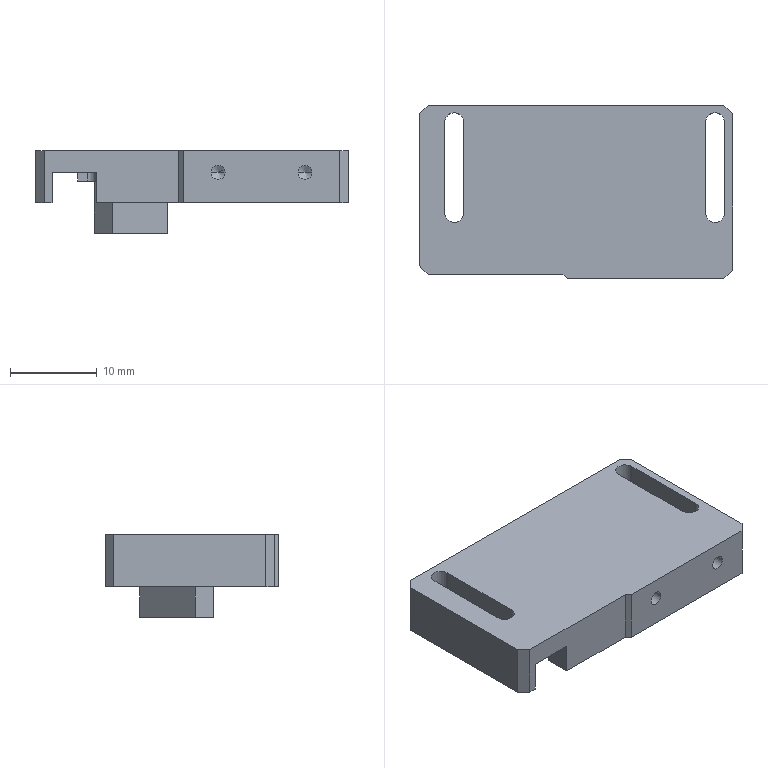CAM job | NX | 3-axis milling | part box 36 x 20 x 9.5 mm | stock box 40 x 24 x 10.5 mm
Tools:
number,name,description,diameter,corner_radius,flute_length,length,flutes
9,D10JING,Milling Tool-5 Parameters,10.0,0.0,50.0,75.0,2
10,D10,Milling Tool-5 Parameters,10.0,0.0,50.0,75.0,2
6,D6,Milling Tool-5 Parameters,6.0,0.0,50.0,75.0,2
2,D2,Milling Tool-5 Parameters,2.0,0.0,50.0,75.0,2
7,D6A45,Milling Tool-5 Parameters,6.0,0.0,3.0,3.0,2
Operations:
program,operation,operation_type,tool,method,geometry_group,spindle_rpm,surface_speed,feed_per_tooth,feed_cut,feed_plunge,cut_length_mm,path_length_mm,cut_time_min,machine_time_min
1,FLOOR_WALL,VolumeBased25DMillingOperation,D10JING,METHOD,A,9500.0,298.0,0.0658,1250.0,100.0,281.997,335.997,0.2256,0.231
1,ZLEVEL_PROFILE,ZLevelMilling,D10,METHOD,A,9500.0,298.0,0.1316,2500.0,1000.0,2752.078,2818.428,1.124,1.13
1,CAVITY_MILL,CavityMilling,D10,METHOD,A,9500.0,298.0,0.1579,3000.0,1000.0,3198.047,3863.307,1.235,1.302
1,CAVITY_MILL_COPY,CavityMilling,D6,METHOD,A,9509.0,179.0,0.0789,1500.0,1000.0,608.15,1362.249,0.4685,0.5439
1,CAVITY_MILL_COPY_COPY,CavityMilling,D2,METHOD,A,9974.0,94.0,0.0501,1000.0,1000.0,2214.844,4126.736,2.215,2.406
1,FLOOR_WALL_2,VolumeBased25DMillingOperation,D2,METHOD,A,9500.0,298.0,0.0658,1250.0,100.0,1113.518,2265.885,0.8908,1.006
1,ZLEVEL_PROFILE_COPY,ZLevelMilling,D2,METHOD,A,9500.0,59.0,0.0526,1000.0,1000.0,791.249,970.309,0.7912,0.8092
1,ZLEVEL_PROFILE_1,ZLevelMilling,D6A45,METHOD,A,9500.0,179.0,0.0658,1250.0,100.0,37.125,95.125,0.0297,0.0355
1,ZLEVEL_PROFILE_1_COPY,ZLevelMilling,D6A45,METHOD,A,9500.0,179.0,0.0658,1250.0,100.0,175.563,411.618,0.1405,0.1641
1,ZLEVEL_PROFILE_1_COPY_COPY,ZLevelMilling,D6A45,METHOD,A,9500.0,179.0,0.0658,1250.0,100.0,49.111,229.226,0.0393,0.0573
1,111,ZLevelMilling,D6,METHOD,A,9500.0,298.0,0.0632,1200.0,1000.0,137.061,211.761,0.1149,0.1224